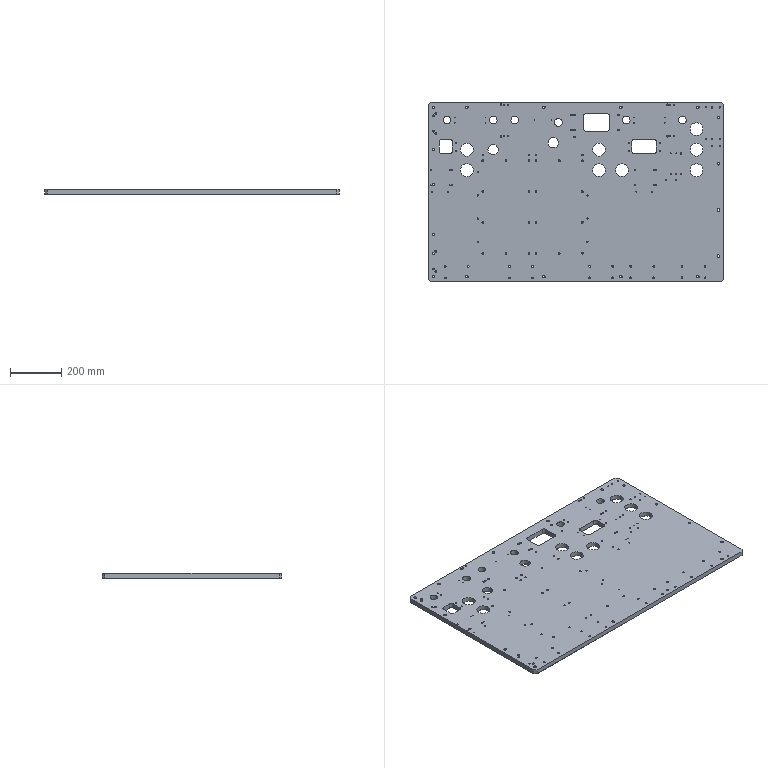Part | NX | 1 solid | 679 faces | box 1149 x 700 x 20 mm | volume 15216652 mm3 | cylinder 362 | cone 274 | plane 43 | commonest cylinder face diameters 6.8 x94 4.2 x60 5 x46 10 x34 16 x34 6 x22